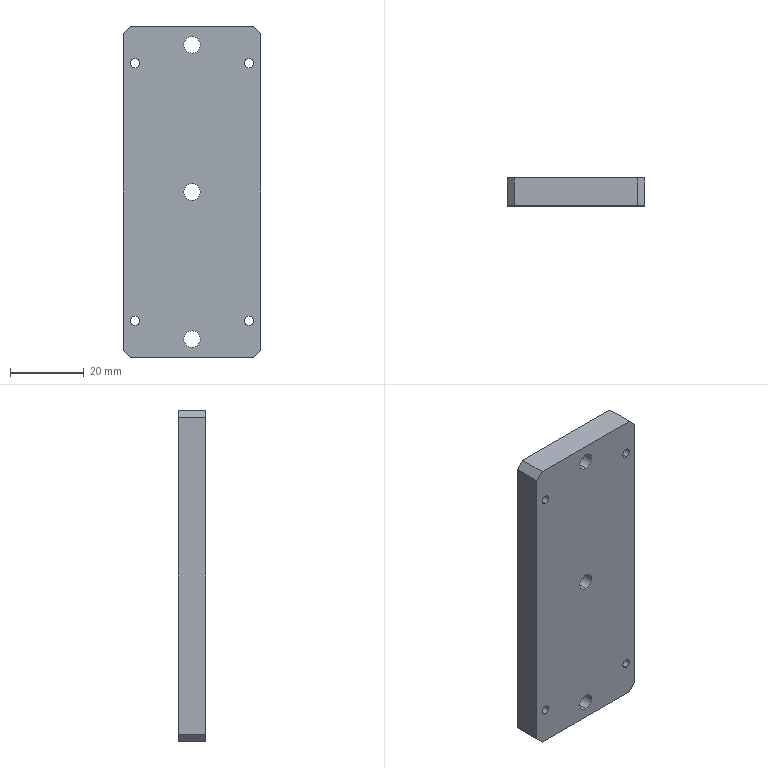Part | STEP file | PN_0032 | 1 solid | 33 faces | box 37.5 x 7.5 x 90 mm | volume 24273 mm3 | cylinder 20 | plane 13 | commonest cylinder face diameters 2.5 x8 4.5 x6 8 x6